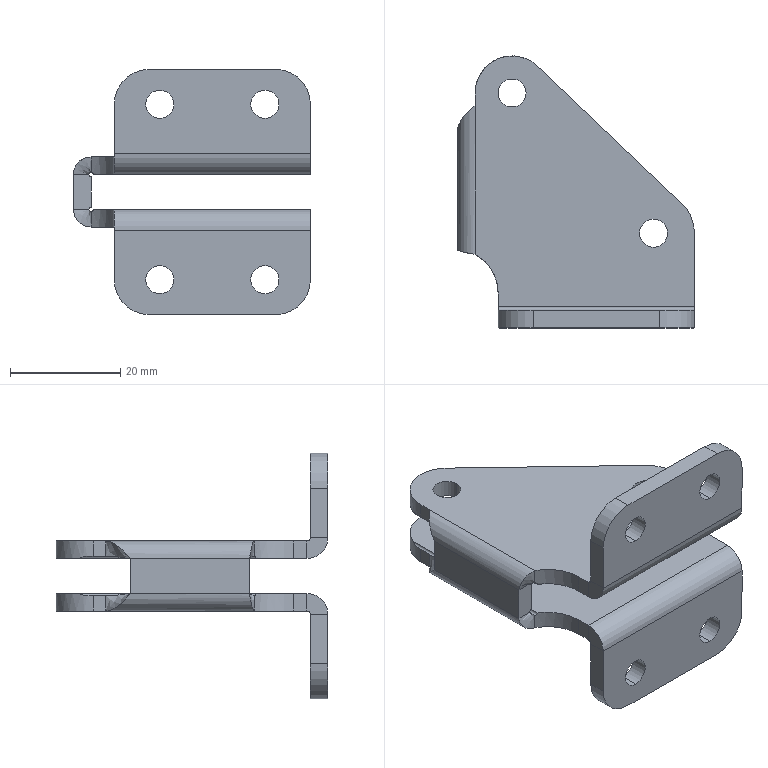Part | SolidWorks | features Cut 5, Fillet 4, Boss 1, Extrusion 1, FlattenBends 1, ProcessBends 1, SheetMetal 1 | 1 solid | 72 faces | box 42.926 x 49.252 x 44.45 mm | volume 12813 mm3 | cylinder 38 | plane 30 | spline 4 | commonest cylinder face diameters 5.08 x16 0.794 x6 12.7 x4 1.27 x2 6.35 x2 7.62 x2